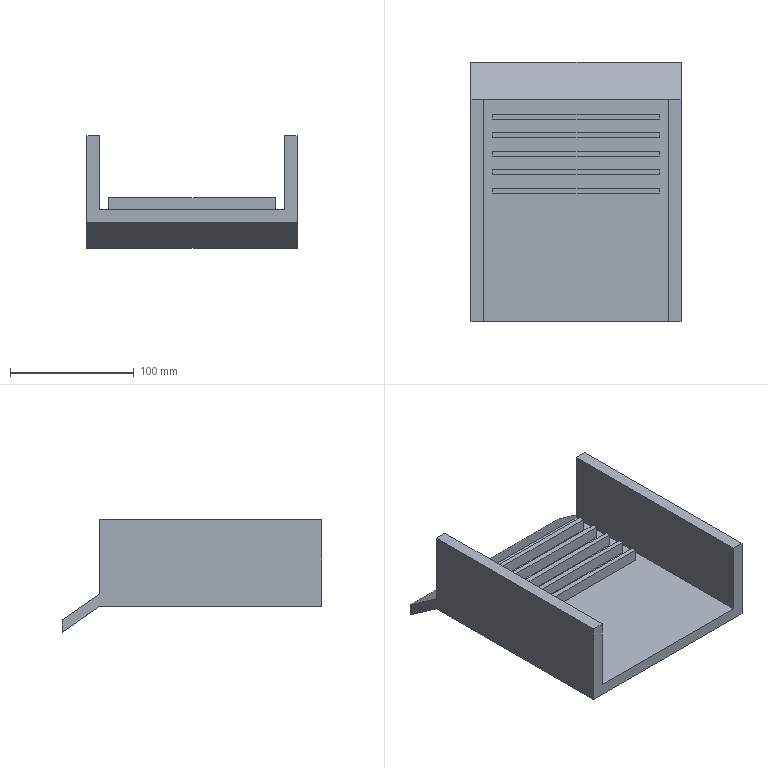Part | SolidWorks | features ICE 3, Extrusion 1, LPattern 1 | 1 solid | 39 faces | box 170 x 210 x 91.006 mm | volume 600000 mm3 | plane 39
STEP:
#1=CARTESIAN_POINT('',(67.5,14.,20.));
#2=VERTEX_POINT('',#1);
#3=CARTESIAN_POINT('',(67.5,18.,20.));
#4=VERTEX_POINT('',#3);
#5=CARTESIAN_POINT('',(67.5,14.,20.));
#6=DIRECTION('',(0.,1.,0.));
#7=VECTOR('',#6,1000.);
#8=LINE('',#5,#7);
#9=EDGE_CURVE('',#2,#4,#8,.T.);
#10=ORIENTED_EDGE('',*,*,#9,.T.);
#11=CARTESIAN_POINT('',(-67.5,18.,20.));
#12=VERTEX_POINT('',#11);
#13=CARTESIAN_POINT('',(-67.5,18.,20.));
#14=DIRECTION('',(-1.,0.,0.));
#15=VECTOR('',#14,1000.);
#16=LINE('',#13,#15);
#17=EDGE_CURVE('',#4,#12,#16,.T.);
#18=ORIENTED_EDGE('',*,*,#17,.T.);
#19=CARTESIAN_POINT('',(-67.5,14.,20.));
#20=VERTEX_POINT('',#19);
#21=CARTESIAN_POINT('',(-67.5,14.,20.));
#22=DIRECTION('',(0.,-1.,0.));
#23=VECTOR('',#22,1000.);
#24=LINE('',#21,#23);
#25=EDGE_CURVE('',#12,#20,#24,.T.);
#26=ORIENTED_EDGE('',*,*,#25,.T.);
#27=CARTESIAN_POINT('',(-67.5,14.,20.));
#28=DIRECTION('',(1.,0.,0.));
#29=VECTOR('',#28,1000.);
#30=LINE('',#27,#29);
#31=EDGE_CURVE('',#20,#2,#30,.T.);
#32=ORIENTED_EDGE('',*,*,#31,.T.);
#33=EDGE_LOOP('',(#10,#18,#26,#32));
#34=FACE_OUTER_BOUND('',#33,.T.);
#35=CARTESIAN_POINT('',(0.,-60.,20.));
#36=DIRECTION('',(0.,0.,-1.));
#37=DIRECTION('',(-1.,0.,0.));
#38=AXIS2_PLACEMENT_3D('',#35,#36,#37);
#39=PLANE('',#38);
#40=ADVANCED_FACE('',(#34),#39,.F.);
#41=CARTESIAN_POINT('',(-67.5,14.,10.));
#42=VERTEX_POINT('',#41);
#43=CARTESIAN_POINT('',(67.5,14.,10.));
#44=VERTEX_POINT('',#43);
#45=CARTESIAN_POINT('',(-67.5,14.,10.));
#46=DIRECTION('',(1.,0.,0.));
#47=VECTOR('',#46,1000.);
#48=LINE('',#45,#47);
#49=EDGE_CURVE('',#42,#44,#48,.T.);
#50=ORIENTED_EDGE('',*,*,#49,.T.);
#51=CARTESIAN_POINT('',(67.5,14.,20.));
#52=DIRECTION('',(0.,0.,-1.));
#53=VECTOR('',#52,1000.);
#54=LINE('',#51,#53);
#55=EDGE_CURVE('',#2,#44,#54,.T.);
#56=ORIENTED_EDGE('',*,*,#55,.F.);
#57=ORIENTED_EDGE('',*,*,#31,.F.);
#58=CARTESIAN_POINT('',(-67.5,14.,20.));
#59=DIRECTION('',(0.,0.,-1.));
#60=VECTOR('',#59,1000.);
#61=LINE('',#58,#60);
#62=EDGE_CURVE('',#20,#42,#61,.T.);
#63=ORIENTED_EDGE('',*,*,#62,.T.);
#64=EDGE_LOOP('',(#50,#56,#57,#63));
#65=FACE_OUTER_BOUND('',#64,.T.);
#66=CARTESIAN_POINT('',(-67.5,14.,20.));
#67=DIRECTION('',(0.,1.,0.));
#68=DIRECTION('',(0.,0.,1.));
#69=AXIS2_PLACEMENT_3D('',#66,#67,#68);
#70=PLANE('',#69);
#71=ADVANCED_FACE('',(#65),#70,.F.);
#72=CARTESIAN_POINT('',(-67.5,18.,10.));
#73=VERTEX_POINT('',#72);
#74=CARTESIAN_POINT('',(-67.5,14.,10.));
#75=DIRECTION('',(0.,-1.,0.));
#76=VECTOR('',#75,1000.);
#77=LINE('',#74,#76);
#78=EDGE_CURVE('',#73,#42,#77,.T.);
#79=ORIENTED_EDGE('',*,*,#78,.T.);
#80=ORIENTED_EDGE('',*,*,#62,.F.);
#81=ORIENTED_EDGE('',*,*,#25,.F.);
#82=CARTESIAN_POINT('',(-67.5,18.,20.));
#83=DIRECTION('',(0.,0.,-1.));
#84=VECTOR('',#83,1000.);
#85=LINE('',#82,#84);
#86=EDGE_CURVE('',#12,#73,#85,.T.);
#87=ORIENTED_EDGE('',*,*,#86,.T.);
#88=EDGE_LOOP('',(#79,#80,#81,#87));
#89=FACE_OUTER_BOUND('',#88,.T.);
#90=CARTESIAN_POINT('',(-67.5,14.,20.));
#91=DIRECTION('',(1.,0.,0.));
#92=DIRECTION('',(0.,0.,-1.));
#93=AXIS2_PLACEMENT_3D('',#90,#91,#92);
#94=PLANE('',#93);
#95=ADVANCED_FACE('',(#89),#94,.F.);
#96=CARTESIAN_POINT('',(67.5,18.,10.));
#97=VERTEX_POINT('',#96);
#98=CARTESIAN_POINT('',(-67.5,18.,10.));
#99=DIRECTION('',(-1.,0.,0.));
#100=VECTOR('',#99,1000.);
#101=LINE('',#98,#100);
#102=EDGE_CURVE('',#97,#73,#101,.T.);
#103=ORIENTED_EDGE('',*,*,#102,.T.);
#104=ORIENTED_EDGE('',*,*,#86,.F.);
#105=ORIENTED_EDGE('',*,*,#17,.F.);
#106=CARTESIAN_POINT('',(67.5,18.,20.));
#107=DIRECTION('',(0.,0.,-1.));
#108=VECTOR('',#107,1000.);
#109=LINE('',#106,#108);
#110=EDGE_CURVE('',#4,#97,#109,.T.);
#111=ORIENTED_EDGE('',*,*,#110,.T.);
#112=EDGE_LOOP('',(#103,#104,#105,#111));
#113=FACE_OUTER_BOUND('',#112,.T.);
#114=CARTESIAN_POINT('',(-67.5,18.,20.));
#115=DIRECTION('',(0.,-1.,0.));
#116=DIRECTION('',(0.,0.,-1.));
#117=AXIS2_PLACEMENT_3D('',#114,#115,#116);
#118=PLANE('',#117);
#119=ADVANCED_FACE('',(#113),#118,.F.);
#120=CARTESIAN_POINT('',(67.5,14.,10.));
#121=DIRECTION('',(0.,1.,0.));
#122=VECTOR('',#121,1000.);
#123=LINE('',#120,#122);
#124=EDGE_CURVE('',#44,#97,#123,.T.);
#125=ORIENTED_EDGE('',*,*,#124,.T.);
#126=ORIENTED_EDGE('',*,*,#110,.F.);
#127=ORIENTED_EDGE('',*,*,#9,.F.);
#128=ORIENTED_EDGE('',*,*,#55,.T.);
#129=EDGE_LOOP('',(#125,#126,#127,#128));
#130=FACE_OUTER_BOUND('',#129,.T.);
#131=CARTESIAN_POINT('',(67.5,14.,20.));
#132=DIRECTION('',(-1.,0.,0.));
#133=DIRECTION('',(0.,0.,1.));
#134=AXIS2_PLACEMENT_3D('',#131,#132,#133);
#135=PLANE('',#134);
#136=ADVANCED_FACE('',(#130),#135,.F.);
#137=CARTESIAN_POINT('',(67.5,29.,20.));
#138=VERTEX_POINT('',#137);
#139=CARTESIAN_POINT('',(67.5,33.,20.));
#140=VERTEX_POINT('',#139);
#141=CARTESIAN_POINT('',(67.5,29.,20.));
#142=DIRECTION('',(0.,1.,0.));
#143=VECTOR('',#142,1000.);
#144=LINE('',#141,#143);
#145=EDGE_CURVE('',#138,#140,#144,.T.);
#146=ORIENTED_EDGE('',*,*,#145,.T.);
#147=CARTESIAN_POINT('',(-67.5,33.,20.));
#148=VERTEX_POINT('',#147);
#149=CARTESIAN_POINT('',(-67.5,33.,20.));
#150=DIRECTION('',(-1.,0.,0.));
#151=VECTOR('',#150,1000.);
#152=LINE('',#149,#151);
#153=EDGE_CURVE('',#140,#148,#152,.T.);
#154=ORIENTED_EDGE('',*,*,#153,.T.);
#155=CARTESIAN_POINT('',(-67.5,29.,20.));
#156=VERTEX_POINT('',#155);
#157=CARTESIAN_POINT('',(-67.5,29.,20.));
#158=DIRECTION('',(0.,-1.,0.));
#159=VECTOR('',#158,1000.);
#160=LINE('',#157,#159);
#161=EDGE_CURVE('',#148,#156,#160,.T.);
#162=ORIENTED_EDGE('',*,*,#161,.T.);
#163=CARTESIAN_POINT('',(-67.5,29.,20.));
#164=DIRECTION('',(1.,0.,0.));
#165=VECTOR('',#164,1000.);
#166=LINE('',#163,#165);
#167=EDGE_CURVE('',#156,#138,#166,.T.);
#168=ORIENTED_EDGE('',*,*,#167,.T.);
#169=EDGE_LOOP('',(#146,#154,#162,#168));
#170=FACE_OUTER_BOUND('',#169,.T.);
#171=CARTESIAN_POINT('',(0.,-45.,20.));
#172=DIRECTION('',(0.,0.,-1.));
#173=DIRECTION('',(-1.,0.,0.));
#174=AXIS2_PLACEMENT_3D('',#171,#172,#173);
#175=PLANE('',#174);
#176=ADVANCED_FACE('',(#170),#175,.F.);
#177=CARTESIAN_POINT('',(-67.5,29.,10.));
#178=VERTEX_POINT('',#177);
#179=CARTESIAN_POINT('',(67.5,29.,10.));
#180=VERTEX_POINT('',#179);
#181=CARTESIAN_POINT('',(-67.5,29.,10.));
#182=DIRECTION('',(1.,0.,0.));
#183=VECTOR('',#182,1000.);
#184=LINE('',#181,#183);
#185=EDGE_CURVE('',#178,#180,#184,.T.);
#186=ORIENTED_EDGE('',*,*,#185,.T.);
#187=CARTESIAN_POINT('',(67.5,29.,20.));
#188=DIRECTION('',(0.,0.,-1.));
#189=VECTOR('',#188,1000.);
#190=LINE('',#187,#189);
#191=EDGE_CURVE('',#138,#180,#190,.T.);
#192=ORIENTED_EDGE('',*,*,#191,.F.);
#193=ORIENTED_EDGE('',*,*,#167,.F.);
#194=CARTESIAN_POINT('',(-67.5,29.,20.));
#195=DIRECTION('',(0.,0.,-1.));
#196=VECTOR('',#195,1000.);
#197=LINE('',#194,#196);
#198=EDGE_CURVE('',#156,#178,#197,.T.);
#199=ORIENTED_EDGE('',*,*,#198,.T.);
#200=EDGE_LOOP('',(#186,#192,#193,#199));
#201=FACE_OUTER_BOUND('',#200,.T.);
#202=CARTESIAN_POINT('',(-67.5,29.,20.));
#203=DIRECTION('',(0.,1.,0.));
#204=DIRECTION('',(0.,0.,1.));
#205=AXIS2_PLACEMENT_3D('',#202,#203,#204);
#206=PLANE('',#205);
#207=ADVANCED_FACE('',(#201),#206,.F.);
#208=CARTESIAN_POINT('',(-67.5,33.,10.));
#209=VERTEX_POINT('',#208);
#210=CARTESIAN_POINT('',(-67.5,29.,10.));
#211=DIRECTION('',(0.,-1.,0.));
#212=VECTOR('',#211,1000.);
#213=LINE('',#210,#212);
#214=EDGE_CURVE('',#209,#178,#213,.T.);
#215=ORIENTED_EDGE('',*,*,#214,.T.);
#216=ORIENTED_EDGE('',*,*,#198,.F.);
#217=ORIENTED_EDGE('',*,*,#161,.F.);
#218=CARTESIAN_POINT('',(-67.5,33.,20.));
#219=DIRECTION('',(0.,0.,-1.));
#220=VECTOR('',#219,1000.);
#221=LINE('',#218,#220);
#222=EDGE_CURVE('',#148,#209,#221,.T.);
#223=ORIENTED_EDGE('',*,*,#222,.T.);
#224=EDGE_LOOP('',(#215,#216,#217,#223));
#225=FACE_OUTER_BOUND('',#224,.T.);
#226=CARTESIAN_POINT('',(-67.5,29.,20.));
#227=DIRECTION('',(1.,0.,0.));
#228=DIRECTION('',(0.,0.,-1.));
#229=AXIS2_PLACEMENT_3D('',#226,#227,#228);
#230=PLANE('',#229);
#231=ADVANCED_FACE('',(#225),#230,.F.);
#232=CARTESIAN_POINT('',(67.5,33.,10.));
#233=VERTEX_POINT('',#232);
#234=CARTESIAN_POINT('',(-67.5,33.,10.));
#235=DIRECTION('',(-1.,0.,0.));
#236=VECTOR('',#235,1000.);
#237=LINE('',#234,#236);
#238=EDGE_CURVE('',#233,#209,#237,.T.);
#239=ORIENTED_EDGE('',*,*,#238,.T.);
#240=ORIENTED_EDGE('',*,*,#222,.F.);
#241=ORIENTED_EDGE('',*,*,#153,.F.);
#242=CARTESIAN_POINT('',(67.5,33.,20.));
#243=DIRECTION('',(0.,0.,-1.));
#244=VECTOR('',#243,1000.);
#245=LINE('',#242,#244);
#246=EDGE_CURVE('',#140,#233,#245,.T.);
#247=ORIENTED_EDGE('',*,*,#246,.T.);
#248=EDGE_LOOP('',(#239,#240,#241,#247));
#249=FACE_OUTER_BOUND('',#248,.T.);
#250=CARTESIAN_POINT('',(-67.5,33.,20.));
#251=DIRECTION('',(0.,-1.,0.));
#252=DIRECTION('',(0.,0.,-1.));
#253=AXIS2_PLACEMENT_3D('',#250,#251,#252);
#254=PLANE('',#253);
#255=ADVANCED_FACE('',(#249),#254,.F.);
#256=CARTESIAN_POINT('',(67.5,29.,10.));
#257=DIRECTION('',(0.,1.,0.));
#258=VECTOR('',#257,1000.);
#259=LINE('',#256,#258);
#260=EDGE_CURVE('',#180,#233,#259,.T.);
#261=ORIENTED_EDGE('',*,*,#260,.T.);
#262=ORIENTED_EDGE('',*,*,#246,.F.);
#263=ORIENTED_EDGE('',*,*,#145,.F.);
#264=ORIENTED_EDGE('',*,*,#191,.T.);
#265=EDGE_LOOP('',(#261,#262,#263,#264));
#266=FACE_OUTER_BOUND('',#265,.T.);
#267=CARTESIAN_POINT('',(67.5,29.,20.));
#268=DIRECTION('',(-1.,0.,0.));
#269=DIRECTION('',(0.,0.,1.));
#270=AXIS2_PLACEMENT_3D('',#267,#268,#269);
#271=PLANE('',#270);
#272=ADVANCED_FACE('',(#266),#271,.F.);
#273=CARTESIAN_POINT('',(67.5,44.,20.));
#274=VERTEX_POINT('',#273);
#275=CARTESIAN_POINT('',(67.5,48.,20.));
#276=VERTEX_POINT('',#275);
#277=CARTESIAN_POINT('',(67.5,44.,20.));
#278=DIRECTION('',(0.,1.,0.));
#279=VECTOR('',#278,1000.);
#280=LINE('',#277,#279);
#281=EDGE_CURVE('',#274,#276,#280,.T.);
#282=ORIENTED_EDGE('',*,*,#281,.T.);
#283=CARTESIAN_POINT('',(-67.5,48.,20.));
#284=VERTEX_POINT('',#283);
#285=CARTESIAN_POINT('',(-67.5,48.,20.));
#286=DIRECTION('',(-1.,0.,0.));
#287=VECTOR('',#286,1000.);
#288=LINE('',#285,#287);
#289=EDGE_CURVE('',#276,#284,#288,.T.);
#290=ORIENTED_EDGE('',*,*,#289,.T.);
#291=CARTESIAN_POINT('',(-67.5,44.,20.));
#292=VERTEX_POINT('',#291);
#293=CARTESIAN_POINT('',(-67.5,44.,20.));
#294=DIRECTION('',(0.,-1.,0.));
#295=VECTOR('',#294,1000.);
#296=LINE('',#293,#295);
#297=EDGE_CURVE('',#284,#292,#296,.T.);
#298=ORIENTED_EDGE('',*,*,#297,.T.);
#299=CARTESIAN_POINT('',(-67.5,44.,20.));
#300=DIRECTION('',(1.,0.,0.));
#301=VECTOR('',#300,1000.);
#302=LINE('',#299,#301);
#303=EDGE_CURVE('',#292,#274,#302,.T.);
#304=ORIENTED_EDGE('',*,*,#303,.T.);
#305=EDGE_LOOP('',(#282,#290,#298,#304));
#306=FACE_OUTER_BOUND('',#305,.T.);
#307=CARTESIAN_POINT('',(0.,-30.,20.));
#308=DIRECTION('',(0.,0.,-1.));
#309=DIRECTION('',(-1.,0.,0.));
#310=AXIS2_PLACEMENT_3D('',#307,#308,#309);
#311=PLANE('',#310);
#312=ADVANCED_FACE('',(#306),#311,.F.);
#313=CARTESIAN_POINT('',(-67.5,44.,10.));
#314=VERTEX_POINT('',#313);
#315=CARTESIAN_POINT('',(67.5,44.,10.));
#316=VERTEX_POINT('',#315);
#317=CARTESIAN_POINT('',(-67.5,44.,10.));
#318=DIRECTION('',(1.,0.,0.));
#319=VECTOR('',#318,1000.);
#320=LINE('',#317,#319);
#321=EDGE_CURVE('',#314,#316,#320,.T.);
#322=ORIENTED_EDGE('',*,*,#321,.T.);
#323=CARTESIAN_POINT('',(67.5,44.,20.));
#324=DIRECTION('',(0.,0.,-1.));
#325=VECTOR('',#324,1000.);
#326=LINE('',#323,#325);
#327=EDGE_CURVE('',#274,#316,#326,.T.);
#328=ORIENTED_EDGE('',*,*,#327,.F.);
#329=ORIENTED_EDGE('',*,*,#303,.F.);
#330=CARTESIAN_POINT('',(-67.5,44.,20.));
#331=DIRECTION('',(0.,0.,-1.));
#332=VECTOR('',#331,1000.);
#333=LINE('',#330,#332);
#334=EDGE_CURVE('',#292,#314,#333,.T.);
#335=ORIENTED_EDGE('',*,*,#334,.T.);
#336=EDGE_LOOP('',(#322,#328,#329,#335));
#337=FACE_OUTER_BOUND('',#336,.T.);
#338=CARTESIAN_POINT('',(-67.5,44.,20.));
#339=DIRECTION('',(0.,1.,0.));
#340=DIRECTION('',(0.,0.,1.));
#341=AXIS2_PLACEMENT_3D('',#338,#339,#340);
#342=PLANE('',#341);
#343=ADVANCED_FACE('',(#337),#342,.F.);
#344=CARTESIAN_POINT('',(-67.5,48.,10.));
#345=VERTEX_POINT('',#344);
#346=CARTESIAN_POINT('',(-67.5,44.,10.));
#347=DIRECTION('',(0.,-1.,0.));
#348=VECTOR('',#347,1000.);
#349=LINE('',#346,#348);
#350=EDGE_CURVE('',#345,#314,#349,.T.);
#351=ORIENTED_EDGE('',*,*,#350,.T.);
#352=ORIENTED_EDGE('',*,*,#334,.F.);
#353=ORIENTED_EDGE('',*,*,#297,.F.);
#354=CARTESIAN_POINT('',(-67.5,48.,20.));
#355=DIRECTION('',(0.,0.,-1.));
#356=VECTOR('',#355,1000.);
#357=LINE('',#354,#356);
#358=EDGE_CURVE('',#284,#345,#357,.T.);
#359=ORIENTED_EDGE('',*,*,#358,.T.);
#360=EDGE_LOOP('',(#351,#352,#353,#359));
#361=FACE_OUTER_BOUND('',#360,.T.);
#362=CARTESIAN_POINT('',(-67.5,44.,20.));
#363=DIRECTION('',(1.,0.,0.));
#364=DIRECTION('',(0.,0.,-1.));
#365=AXIS2_PLACEMENT_3D('',#362,#363,#364);
#366=PLANE('',#365);
#367=ADVANCED_FACE('',(#361),#366,.F.);
#368=CARTESIAN_POINT('',(67.5,48.,10.));
#369=VERTEX_POINT('',#368);
#370=CARTESIAN_POINT('',(-67.5,48.,10.));
#371=DIRECTION('',(-1.,0.,0.));
#372=VECTOR('',#371,1000.);
#373=LINE('',#370,#372);
#374=EDGE_CURVE('',#369,#345,#373,.T.);
#375=ORIENTED_EDGE('',*,*,#374,.T.);
#376=ORIENTED_EDGE('',*,*,#358,.F.);
#377=ORIENTED_EDGE('',*,*,#289,.F.);
#378=CARTESIAN_POINT('',(67.5,48.,20.));
#379=DIRECTION('',(0.,0.,-1.));
#380=VECTOR('',#379,1000.);
#381=LINE('',#378,#380);
#382=EDGE_CURVE('',#276,#369,#381,.T.);
#383=ORIENTED_EDGE('',*,*,#382,.T.);
#384=EDGE_LOOP('',(#375,#376,#377,#383));
#385=FACE_OUTER_BOUND('',#384,.T.);
#386=CARTESIAN_POINT('',(-67.5,48.,20.));
#387=DIRECTION('',(0.,-1.,0.));
#388=DIRECTION('',(0.,0.,-1.));
#389=AXIS2_PLACEMENT_3D('',#386,#387,#388);
#390=PLANE('',#389);
#391=ADVANCED_FACE('',(#385),#390,.F.);
#392=CARTESIAN_POINT('',(67.5,44.,10.));
#393=DIRECTION('',(0.,1.,0.));
#394=VECTOR('',#393,1000.);
#395=LINE('',#392,#394);
#396=EDGE_CURVE('',#316,#369,#395,.T.);
#397=ORIENTED_EDGE('',*,*,#396,.T.);
#398=ORIENTED_EDGE('',*,*,#382,.F.);
#399=ORIENTED_EDGE('',*,*,#281,.F.);
#400=ORIENTED_EDGE('',*,*,#327,.T.);
#401=EDGE_LOOP('',(#397,#398,#399,#400));
#402=FACE_OUTER_BOUND('',#401,.T.);
#403=CARTESIAN_POINT('',(67.5,44.,20.));
#404=DIRECTION('',(-1.,0.,0.));
#405=DIRECTION('',(0.,0.,1.));
#406=AXIS2_PLACEMENT_3D('',#403,#404,#405);
#407=PLANE('',#406);
#408=ADVANCED_FACE('',(#402),#407,.F.);
#409=CARTESIAN_POINT('',(67.5,74.,10.));
#410=VERTEX_POINT('',#409);
#411=CARTESIAN_POINT('',(67.5,78.,10.));
#412=VERTEX_POINT('',#411);
#413=CARTESIAN_POINT('',(67.5,74.,10.));
#414=DIRECTION('',(0.,1.,0.));
#415=VECTOR('',#414,1000.);
#416=LINE('',#413,#415);
#417=EDGE_CURVE('',#410,#412,#416,.T.);
#418=ORIENTED_EDGE('',*,*,#417,.F.);
#419=CARTESIAN_POINT('',(-67.5,74.,10.));
#420=VERTEX_POINT('',#419);
#421=CARTESIAN_POINT('',(-67.5,74.,10.));
#422=DIRECTION('',(1.,0.,0.));
#423=VECTOR('',#422,1000.);
#424=LINE('',#421,#423);
#425=EDGE_CURVE('',#420,#410,#424,.T.);
#426=ORIENTED_EDGE('',*,*,#425,.F.);
#427=CARTESIAN_POINT('',(-67.5,78.,10.));
#428=VERTEX_POINT('',#427);
#429=CARTESIAN_POINT('',(-67.5,74.,10.));
#430=DIRECTION('',(0.,-1.,0.));
#431=VECTOR('',#430,1000.);
#432=LINE('',#429,#431);
#433=EDGE_CURVE('',#428,#420,#432,.T.);
#434=ORIENTED_EDGE('',*,*,#433,.F.);
#435=CARTESIAN_POINT('',(-67.5,78.,10.));
#436=DIRECTION('',(-1.,0.,0.));
#437=VECTOR('',#436,1000.);
#438=LINE('',#435,#437);
#439=EDGE_CURVE('',#412,#428,#438,.T.);
#440=ORIENTED_EDGE('',*,*,#439,.F.);
#441=EDGE_LOOP('',(#418,#426,#434,#440));
#442=FACE_BOUND('',#441,.T.);
#443=CARTESIAN_POINT('',(75.,90.,10.));
#444=VERTEX_POINT('',#443);
#445=CARTESIAN_POINT('',(75.,-90.,10.));
#446=VERTEX_POINT('',#445);
#447=CARTESIAN_POINT('',(75.,90.,10.));
#448=DIRECTION('',(0.,-1.,0.));
#449=VECTOR('',#448,1000.);
#450=LINE('',#447,#449);
#451=EDGE_CURVE('',#444,#446,#450,.T.);
#452=ORIENTED_EDGE('',*,*,#451,.F.);
#453=CARTESIAN_POINT('',(-75.,90.,10.));
#454=VERTEX_POINT('',#453);
#455=CARTESIAN_POINT('',(-85.,90.,10.));
#456=DIRECTION('',(-1.,0.,0.));
#457=VECTOR('',#456,1000.);
#458=LINE('',#455,#457);
#459=EDGE_CURVE('',#444,#454,#458,.T.);
#460=ORIENTED_EDGE('',*,*,#459,.T.);
#461=CARTESIAN_POINT('',(-75.,-90.,10.));
#462=VERTEX_POINT('',#461);
#463=CARTESIAN_POINT('',(-75.,90.,10.));
#464=DIRECTION('',(0.,1.,0.));
#465=VECTOR('',#464,1000.);
#466=LINE('',#463,#465);
#467=EDGE_CURVE('',#462,#454,#466,.T.);
#468=ORIENTED_EDGE('',*,*,#467,.F.);
#469=CARTESIAN_POINT('',(-85.,-90.,10.));
#470=DIRECTION('',(1.,0.,0.));
#471=VECTOR('',#470,1000.);
#472=LINE('',#469,#471);
#473=EDGE_CURVE('',#462,#446,#472,.T.);
#474=ORIENTED_EDGE('',*,*,#473,.T.);
#475=EDGE_LOOP('',(#452,#460,#468,#474));
#476=FACE_OUTER_BOUND('',#475,.T.);
#477=CARTESIAN_POINT('',(67.5,59.,10.));
#478=VERTEX_POINT('',#477);
#479=CARTESIAN_POINT('',(67.5,63.,10.));
#480=VERTEX_POINT('',#479);
#481=CARTESIAN_POINT('',(67.5,59.,10.));
#482=DIRECTION('',(0.,1.,0.));
#483=VECTOR('',#482,1000.);
#484=LINE('',#481,#483);
#485=EDGE_CURVE('',#478,#480,#484,.T.);
#486=ORIENTED_EDGE('',*,*,#485,.F.);
#487=CARTESIAN_POINT('',(-67.5,59.,10.));
#488=VERTEX_POINT('',#487);
#489=CARTESIAN_POINT('',(-67.5,59.,10.));
#490=DIRECTION('',(1.,0.,0.));
#491=VECTOR('',#490,1000.);
#492=LINE('',#489,#491);
#493=EDGE_CURVE('',#488,#478,#492,.T.);
#494=ORIENTED_EDGE('',*,*,#493,.F.);
#495=CARTESIAN_POINT('',(-67.5,63.,10.));
#496=VERTEX_POINT('',#495);
#497=CARTESIAN_POINT('',(-67.5,59.,10.));
#498=DIRECTION('',(0.,-1.,0.));
#499=VECTOR('',#498,1000.);
#500=LINE('',#497,#499);
#501=EDGE_CURVE('',#496,#488,#500,.T.);
#502=ORIENTED_EDGE('',*,*,#501,.F.);
#503=CARTESIAN_POINT('',(-67.5,63.,10.));
#504=DIRECTION('',(-1.,0.,0.));
#505=VECTOR('',#504,1000.);
#506=LINE('',#503,#505);
#507=EDGE_CURVE('',#480,#496,#506,.T.);
#508=ORIENTED_EDGE('',*,*,#507,.F.);
#509=EDGE_LOOP('',(#486,#494,#502,#508));
#510=FACE_BOUND('',#509,.T.);
#511=ORIENTED_EDGE('',*,*,#396,.F.);
#512=ORIENTED_EDGE('',*,*,#321,.F.);
#513=ORIENTED_EDGE('',*,*,#350,.F.);
#514=ORIENTED_EDGE('',*,*,#374,.F.);
#515=EDGE_LOOP('',(#511,#512,#513,#514));
#516=FACE_BOUND('',#515,.T.);
#517=ORIENTED_EDGE('',*,*,#260,.F.);
#518=ORIENTED_EDGE('',*,*,#185,.F.);
#519=ORIENTED_EDGE('',*,*,#214,.F.);
#520=ORIENTED_EDGE('',*,*,#238,.F.);
#521=EDGE_LOOP('',(#517,#518,#519,#520));
#522=FACE_BOUND('',#521,.T.);
#523=ORIENTED_EDGE('',*,*,#124,.F.);
#524=ORIENTED_EDGE('',*,*,#49,.F.);
#525=ORIENTED_EDGE('',*,*,#78,.F.);
#526=ORIENTED_EDGE('',*,*,#102,.F.);
#527=EDGE_LOOP('',(#523,#524,#525,#526));
#528=FACE_BOUND('',#527,.T.);
#529=CARTESIAN_POINT('',(0.,0.,10.));
#530=DIRECTION('',(0.,0.,-1.));
#531=DIRECTION('',(-1.,0.,0.));
#532=AXIS2_PLACEMENT_3D('',#529,#530,#531);
#533=PLANE('',#532);
#534=ADVANCED_FACE('',(#442,#476,#510,#516,#522,#528),#533,.F.);
#535=CARTESIAN_POINT('',(-85.,90.,10.));
#536=VERTEX_POINT('',#535);
#537=CARTESIAN_POINT('',(-128.144,90.,10.));
#538=DIRECTION('',(1.,0.,0.));
#539=VECTOR('',#538,1000.);
#540=LINE('',#537,#539);
#541=EDGE_CURVE('',#536,#454,#540,.T.);
#542=ORIENTED_EDGE('',*,*,#541,.F.);
#543=CARTESIAN_POINT('',(-85.,90.,70.));
#544=VERTEX_POINT('',#543);
#545=CARTESIAN_POINT('',(-85.,90.,10.));
#546=DIRECTION('',(0.,0.,-1.));
#547=VECTOR('',#546,1000.);
#548=LINE('',#545,#547);
#549=EDGE_CURVE('',#544,#536,#548,.T.);
#550=ORIENTED_EDGE('',*,*,#549,.F.);
#551=CARTESIAN_POINT('',(-75.,90.,70.));
#552=VERTEX_POINT('',#551);
#553=CARTESIAN_POINT('',(-85.,90.,70.));
#554=DIRECTION('',(-1.,0.,0.));
#555=VECTOR('',#554,1000.);
#556=LINE('',#553,#555);
#557=EDGE_CURVE('',#552,#544,#556,.T.);
#558=ORIENTED_EDGE('',*,*,#557,.F.);
#559=CARTESIAN_POINT('',(-75.,90.,70.));
#560=DIRECTION('',(0.,0.,-1.));
#561=VECTOR('',#560,1000.);
#562=LINE('',#559,#561);
#563=EDGE_CURVE('',#552,#454,#562,.T.);
#564=ORIENTED_EDGE('',*,*,#563,.T.);
#565=EDGE_LOOP('',(#542,#550,#558,#564));
#566=FACE_OUTER_BOUND('',#565,.T.);
#567=CARTESIAN_POINT('',(-85.,90.,10.));
#568=DIRECTION('',(0.,-1.,0.));
#569=DIRECTION('',(0.,0.,-1.));
#570=AXIS2_PLACEMENT_3D('',#567,#568,#569);
#571=PLANE('',#570);
#572=ADVANCED_FACE('',(#566),#571,.F.);
#573=CARTESIAN_POINT('',(85.,90.,10.));
#574=VERTEX_POINT('',#573);
#575=CARTESIAN_POINT('',(-128.144,90.,10.));
#576=DIRECTION('',(1.,0.,0.));
#577=VECTOR('',#576,1000.);
#578=LINE('',#575,#577);
#579=EDGE_CURVE('',#444,#574,#578,.T.);
#580=ORIENTED_EDGE('',*,*,#579,.F.);
#581=CARTESIAN_POINT('',(75.,90.,70.));
#582=VERTEX_POINT('',#581);
#583=CARTESIAN_POINT('',(75.,90.,70.));
#584=DIRECTION('',(0.,0.,-1.));
#585=VECTOR('',#584,1000.);
#586=LINE('',#583,#585);
#587=EDGE_CURVE('',#582,#444,#586,.T.);
#588=ORIENTED_EDGE('',*,*,#587,.F.);
#589=CARTESIAN_POINT('',(85.,90.,70.));
#590=VERTEX_POINT('',#589);
#591=CARTESIAN_POINT('',(85.,90.,70.));
#592=DIRECTION('',(-1.,0.,0.));
#593=VECTOR('',#592,1000.);
#594=LINE('',#591,#593);
#595=EDGE_CURVE('',#590,#582,#594,.T.);
#596=ORIENTED_EDGE('',*,*,#595,.F.);
#597=CARTESIAN_POINT('',(85.,90.,10.));
#598=DIRECTION('',(0.,0.,-1.));
#599=VECTOR('',#598,1000.);
#600=LINE('',#597,#599);
#601=EDGE_CURVE('',#590,#574,#600,.T.);
#602=ORIENTED_EDGE('',*,*,#601,.T.);
#603=EDGE_LOOP('',(#580,#588,#596,#602));
#604=FACE_OUTER_BOUND('',#603,.T.);
#605=CARTESIAN_POINT('',(-85.,90.,10.));
#606=DIRECTION('',(0.,-1.,0.));
#607=DIRECTION('',(0.,0.,-1.));
#608=AXIS2_PLACEMENT_3D('',#605,#606,#607);
#609=PLANE('',#608);
#610=ADVANCED_FACE('',(#604),#609,.F.);
#611=CARTESIAN_POINT('',(85.,-90.,0.));
#612=VERTEX_POINT('',#611);
#613=CARTESIAN_POINT('',(85.,90.,0.));
#614=VERTEX_POINT('',#613);
#615=CARTESIAN_POINT('',(85.,-90.,0.));
#616=DIRECTION('',(0.,1.,0.));
#617=VECTOR('',#616,1000.);
#618=LINE('',#615,#617);
#619=EDGE_CURVE('',#612,#614,#618,.T.);
#620=ORIENTED_EDGE('',*,*,#619,.T.);
#621=CARTESIAN_POINT('',(85.,120.,-21.006));
#622=VERTEX_POINT('',#621);
#623=CARTESIAN_POINT('',(85.,90.,0.));
#624=DIRECTION('',(0.,0.8192,-0.5736));
#625=VECTOR('',#624,1000.);
#626=LINE('',#623,#625);
#627=EDGE_CURVE('',#614,#622,#626,.T.);
#628=ORIENTED_EDGE('',*,*,#627,.T.);
#629=CARTESIAN_POINT('',(85.,120.,-11.006));
#630=VERTEX_POINT('',#629);
#631=CARTESIAN_POINT('',(85.,120.,-21.006));
#632=DIRECTION('',(0.,0.,1.));
#633=VECTOR('',#632,1000.);
#634=LINE('',#631,#633);
#635=EDGE_CURVE('',#622,#630,#634,.T.);
#636=ORIENTED_EDGE('',*,*,#635,.T.);
#637=CARTESIAN_POINT('',(85.,120.,-11.006));
#638=DIRECTION('',(0.,-0.8192,0.5736));
#639=VECTOR('',#638,1000.);
#640=LINE('',#637,#639);
#641=EDGE_CURVE('',#630,#574,#640,.T.);
#642=ORIENTED_EDGE('',*,*,#641,.T.);
#643=ORIENTED_EDGE('',*,*,#601,.F.);
#644=CARTESIAN_POINT('',(85.,-90.,70.));
#645=VERTEX_POINT('',#644);
#646=CARTESIAN_POINT('',(85.,90.,70.));
#647=DIRECTION('',(0.,1.,0.));
#648=VECTOR('',#647,1000.);
#649=LINE('',#646,#648);
#650=EDGE_CURVE('',#645,#590,#649,.T.);
#651=ORIENTED_EDGE('',*,*,#650,.F.);
#652=CARTESIAN_POINT('',(85.,-90.,10.));
#653=DIRECTION('',(0.,0.,-1.));
#654=VECTOR('',#653,1000.);
#655=LINE('',#652,#654);
#656=EDGE_CURVE('',#645,#612,#655,.T.);
#657=ORIENTED_EDGE('',*,*,#656,.T.);
#658=EDGE_LOOP('',(#620,#628,#636,#642,#643,#651,#657));
#659=FACE_OUTER_BOUND('',#658,.T.);
#660=CARTESIAN_POINT('',(85.,-90.,10.));
#661=DIRECTION('',(-1.,0.,0.));
#662=DIRECTION('',(0.,0.,1.));
#663=AXIS2_PLACEMENT_3D('',#660,#661,#662);
#664=PLANE('',#663);
#665=ADVANCED_FACE('',(#659),#664,.F.);
#666=CARTESIAN_POINT('',(-85.,90.,0.));
#667=VERTEX_POINT('',#666);
#668=CARTESIAN_POINT('',(-85.,-90.,0.));
#669=VERTEX_POINT('',#668);
#670=CARTESIAN_POINT('',(-85.,-90.,0.));
#671=DIRECTION('',(0.,-1.,0.));
#672=VECTOR('',#671,1000.);
#673=LINE('',#670,#672);
#674=EDGE_CURVE('',#667,#669,#673,.T.);
#675=ORIENTED_EDGE('',*,*,#674,.T.);
#676=CARTESIAN_POINT('',(-85.,-90.,70.));
#677=VERTEX_POINT('',#676);
#678=CARTESIAN_POINT('',(-85.,-90.,10.));
#679=DIRECTION('',(0.,0.,-1.));
#680=VECTOR('',#679,1000.);
#681=LINE('',#678,#680);
#682=EDGE_CURVE('',#677,#669,#681,.T.);
#683=ORIENTED_EDGE('',*,*,#682,.F.);
#684=CARTESIAN_POINT('',(-85.,90.,70.));
#685=DIRECTION('',(0.,-1.,0.));
#686=VECTOR('',#685,1000.);
#687=LINE('',#684,#686);
#688=EDGE_CURVE('',#544,#677,#687,.T.);
#689=ORIENTED_EDGE('',*,*,#688,.F.);
#690=ORIENTED_EDGE('',*,*,#549,.T.);
#691=CARTESIAN_POINT('',(-85.,120.,-11.006));
#692=VERTEX_POINT('',#691);
#693=CARTESIAN_POINT('',(-85.,120.,-11.006));
#694=DIRECTION('',(0.,0.8192,-0.5736));
#695=VECTOR('',#694,1000.);
#696=LINE('',#693,#695);
#697=EDGE_CURVE('',#536,#692,#696,.T.);
#698=ORIENTED_EDGE('',*,*,#697,.T.);
#699=CARTESIAN_POINT('',(-85.,120.,-21.006));
#700=VERTEX_POINT('',#699);
#701=CARTESIAN_POINT('',(-85.,120.,-21.006));
#702=DIRECTION('',(0.,0.,-1.));
#703=VECTOR('',#702,1000.);
#704=LINE('',#701,#703);
#705=EDGE_CURVE('',#692,#700,#704,.T.);
#706=ORIENTED_EDGE('',*,*,#705,.T.);
#707=CARTESIAN_POINT('',(-85.,90.,0.));
#708=DIRECTION('',(0.,-0.8192,0.5736));
#709=VECTOR('',#708,1000.);
#710=LINE('',#707,#709);
#711=EDGE_CURVE('',#700,#667,#710,.T.);
#712=ORIENTED_EDGE('',*,*,#711,.T.);
#713=EDGE_LOOP('',(#675,#683,#689,#690,#698,#706,#712));
#714=FACE_OUTER_BOUND('',#713,.T.);
#715=CARTESIAN_POINT('',(-85.,-90.,10.));
#716=DIRECTION('',(1.,0.,0.));
#717=DIRECTION('',(0.,0.,-1.));
#718=AXIS2_PLACEMENT_3D('',#715,#716,#717);
#719=PLANE('',#718);
#720=ADVANCED_FACE('',(#714),#719,.F.);
#721=CARTESIAN_POINT('',(-85.,-90.,0.));
#722=DIRECTION('',(1.,0.,0.));
#723=VECTOR('',#722,1000.);
#724=LINE('',#721,#723);
#725=EDGE_CURVE('',#669,#612,#724,.T.);
#726=ORIENTED_EDGE('',*,*,#725,.T.);
#727=ORIENTED_EDGE('',*,*,#656,.F.);
#728=CARTESIAN_POINT('',(75.,-90.,70.));
#729=VERTEX_POINT('',#728);
#730=CARTESIAN_POINT('',(85.,-90.,70.));
#731=DIRECTION('',(1.,0.,0.));
#732=VECTOR('',#731,1000.);
#733=LINE('',#730,#732);
#734=EDGE_CURVE('',#729,#645,#733,.T.);
#735=ORIENTED_EDGE('',*,*,#734,.F.);
#736=CARTESIAN_POINT('',(75.,-90.,70.));
#737=DIRECTION('',(0.,0.,-1.));
#738=VECTOR('',#737,1000.);
#739=LINE('',#736,#738);
#740=EDGE_CURVE('',#729,#446,#739,.T.);
#741=ORIENTED_EDGE('',*,*,#740,.T.);
#742=ORIENTED_EDGE('',*,*,#473,.F.);
#743=CARTESIAN_POINT('',(-75.,-90.,70.));
#744=VERTEX_POINT('',#743);
#745=CARTESIAN_POINT('',(-75.,-90.,70.));
#746=DIRECTION('',(0.,0.,-1.));
#747=VECTOR('',#746,1000.);
#748=LINE('',#745,#747);
#749=EDGE_CURVE('',#744,#462,#748,.T.);
#750=ORIENTED_EDGE('',*,*,#749,.F.);
#751=CARTESIAN_POINT('',(-85.,-90.,70.));
#752=DIRECTION('',(1.,0.,0.));
#753=VECTOR('',#752,1000.);
#754=LINE('',#751,#753);
#755=EDGE_CURVE('',#677,#744,#754,.T.);
#756=ORIENTED_EDGE('',*,*,#755,.F.);
#757=ORIENTED_EDGE('',*,*,#682,.T.);
#758=EDGE_LOOP('',(#726,#727,#735,#741,#742,#750,#756,#757));
#759=FACE_OUTER_BOUND('',#758,.T.);
#760=CARTESIAN_POINT('',(-85.,-90.,10.));
#761=DIRECTION('',(0.,1.,0.));
#762=DIRECTION('',(0.,0.,1.));
#763=AXIS2_PLACEMENT_3D('',#760,#761,#762);
#764=PLANE('',#763);
#765=ADVANCED_FACE('',(#759),#764,.F.);
#766=ORIENTED_EDGE('',*,*,#619,.F.);
#767=ORIENTED_EDGE('',*,*,#725,.F.);
#768=ORIENTED_EDGE('',*,*,#674,.F.);
#769=CARTESIAN_POINT('',(-85.,90.,0.));
#770=DIRECTION('',(-1.,0.,0.));
#771=VECTOR('',#770,1000.);
#772=LINE('',#769,#771);
#773=EDGE_CURVE('',#614,#667,#772,.T.);
#774=ORIENTED_EDGE('',*,*,#773,.F.);
#775=EDGE_LOOP('',(#766,#767,#768,#774));
#776=FACE_OUTER_BOUND('',#775,.T.);
#777=CARTESIAN_POINT('',(0.,0.,0.));
#778=DIRECTION('',(0.,0.,-1.));
#779=DIRECTION('',(-1.,0.,0.));
#780=AXIS2_PLACEMENT_3D('',#777,#778,#779);
#781=PLANE('',#780);
#782=ADVANCED_FACE('',(#776),#781,.T.);
#783=ORIENTED_EDGE('',*,*,#467,.T.);
#784=ORIENTED_EDGE('',*,*,#563,.F.);
#785=CARTESIAN_POINT('',(-75.,90.,70.));
#786=DIRECTION('',(0.,1.,0.));
#787=VECTOR('',#786,1000.);
#788=LINE('',#785,#787);
#789=EDGE_CURVE('',#744,#552,#788,.T.);
#790=ORIENTED_EDGE('',*,*,#789,.F.);
#791=ORIENTED_EDGE('',*,*,#749,.T.);
#792=EDGE_LOOP('',(#783,#784,#790,#791));
#793=FACE_OUTER_BOUND('',#792,.T.);
#794=CARTESIAN_POINT('',(-75.,90.,70.));
#795=DIRECTION('',(-1.,0.,0.));
#796=DIRECTION('',(0.,-1.,0.));
#797=AXIS2_PLACEMENT_3D('',#794,#795,#796);
#798=PLANE('',#797);
#799=ADVANCED_FACE('',(#793),#798,.F.);
#800=ORIENTED_EDGE('',*,*,#688,.T.);
#801=ORIENTED_EDGE('',*,*,#755,.T.);
#802=ORIENTED_EDGE('',*,*,#789,.T.);
#803=ORIENTED_EDGE('',*,*,#557,.T.);
#804=EDGE_LOOP('',(#800,#801,#802,#803));
#805=FACE_OUTER_BOUND('',#804,.T.);
#806=CARTESIAN_POINT('',(0.,0.,70.));
#807=DIRECTION('',(0.,0.,1.));
#808=DIRECTION('',(1.,0.,0.));
#809=AXIS2_PLACEMENT_3D('',#806,#807,#808);
#810=PLANE('',#809);
#811=ADVANCED_FACE('',(#805),#810,.T.);
#812=ORIENTED_EDGE('',*,*,#451,.T.);
#813=ORIENTED_EDGE('',*,*,#740,.F.);
#814=CARTESIAN_POINT('',(75.,90.,70.));
#815=DIRECTION('',(0.,-1.,0.));
#816=VECTOR('',#815,1000.);
#817=LINE('',#814,#816);
#818=EDGE_CURVE('',#582,#729,#817,.T.);
#819=ORIENTED_EDGE('',*,*,#818,.F.);
#820=ORIENTED_EDGE('',*,*,#587,.T.);
#821=EDGE_LOOP('',(#812,#813,#819,#820));
#822=FACE_OUTER_BOUND('',#821,.T.);
#823=CARTESIAN_POINT('',(75.,90.,70.));
#824=DIRECTION('',(1.,0.,0.));
#825=DIRECTION('',(0.,1.,0.));
#826=AXIS2_PLACEMENT_3D('',#823,#824,#825);
#827=PLANE('',#826);
#828=ADVANCED_FACE('',(#822),#827,.F.);
#829=ORIENTED_EDGE('',*,*,#650,.T.);
#830=ORIENTED_EDGE('',*,*,#595,.T.);
#831=ORIENTED_EDGE('',*,*,#818,.T.);
#832=ORIENTED_EDGE('',*,*,#734,.T.);
#833=EDGE_LOOP('',(#829,#830,#831,#832));
#834=FACE_OUTER_BOUND('',#833,.T.);
#835=CARTESIAN_POINT('',(0.,0.,70.));
#836=DIRECTION('',(0.,0.,-1.));
#837=DIRECTION('',(-1.,0.,0.));
#838=AXIS2_PLACEMENT_3D('',#835,#836,#837);
#839=PLANE('',#838);
#840=ADVANCED_FACE('',(#834),#839,.F.);
#841=ORIENTED_EDGE('',*,*,#697,.F.);
#842=ORIENTED_EDGE('',*,*,#541,.T.);
#843=ORIENTED_EDGE('',*,*,#459,.F.);
#844=ORIENTED_EDGE('',*,*,#579,.T.);
#845=ORIENTED_EDGE('',*,*,#641,.F.);
#846=CARTESIAN_POINT('',(-128.144,120.,-11.006));
#847=DIRECTION('',(1.,0.,0.));
#848=VECTOR('',#847,1000.);
#849=LINE('',#846,#848);
#850=EDGE_CURVE('',#692,#630,#849,.T.);
#851=ORIENTED_EDGE('',*,*,#850,.F.);
#852=EDGE_LOOP('',(#841,#842,#843,#844,#845,#851));
#853=FACE_OUTER_BOUND('',#852,.T.);
#854=CARTESIAN_POINT('',(-128.144,120.,-11.006));
#855=DIRECTION('',(0.,0.5736,0.8192));
#856=DIRECTION('',(0.,-0.8192,0.5736));
#857=AXIS2_PLACEMENT_3D('',#854,#855,#856);
#858=PLANE('',#857);
#859=ADVANCED_FACE('',(#853),#858,.T.);
#860=ORIENTED_EDGE('',*,*,#705,.F.);
#861=ORIENTED_EDGE('',*,*,#850,.T.);
#862=ORIENTED_EDGE('',*,*,#635,.F.);
#863=CARTESIAN_POINT('',(-128.144,120.,-21.006));
#864=DIRECTION('',(1.,0.,0.));
#865=VECTOR('',#864,1000.);
#866=LINE('',#863,#865);
#867=EDGE_CURVE('',#700,#622,#866,.T.);
#868=ORIENTED_EDGE('',*,*,#867,.F.);
#869=EDGE_LOOP('',(#860,#861,#862,#868));
#870=FACE_OUTER_BOUND('',#869,.T.);
#871=CARTESIAN_POINT('',(-128.144,120.,-21.006));
#872=DIRECTION('',(0.,1.,0.));
#873=DIRECTION('',(0.,0.,1.));
#874=AXIS2_PLACEMENT_3D('',#871,#872,#873);
#875=PLANE('',#874);
#876=ADVANCED_FACE('',(#870),#875,.T.);
#877=ORIENTED_EDGE('',*,*,#711,.F.);
#878=ORIENTED_EDGE('',*,*,#867,.T.);
#879=ORIENTED_EDGE('',*,*,#627,.F.);
#880=ORIENTED_EDGE('',*,*,#773,.T.);
#881=EDGE_LOOP('',(#877,#878,#879,#880));
#882=FACE_OUTER_BOUND('',#881,.T.);
#883=CARTESIAN_POINT('',(-128.144,90.,0.));
#884=DIRECTION('',(0.,-0.5736,-0.8192));
#885=DIRECTION('',(0.,0.8192,-0.5736));
#886=AXIS2_PLACEMENT_3D('',#883,#884,#885);
#887=PLANE('',#886);
#888=ADVANCED_FACE('',(#882),#887,.T.);
#889=ORIENTED_EDGE('',*,*,#417,.T.);
#890=CARTESIAN_POINT('',(67.5,78.,20.));
#891=VERTEX_POINT('',#890);
#892=CARTESIAN_POINT('',(67.5,78.,20.));
#893=DIRECTION('',(0.,0.,-1.));
#894=VECTOR('',#893,1000.);
#895=LINE('',#892,#894);
#896=EDGE_CURVE('',#891,#412,#895,.T.);
#897=ORIENTED_EDGE('',*,*,#896,.F.);
#898=CARTESIAN_POINT('',(67.5,74.,20.));
#899=VERTEX_POINT('',#898);
#900=CARTESIAN_POINT('',(67.5,74.,20.));
#901=DIRECTION('',(0.,1.,0.));
#902=VECTOR('',#901,1000.);
#903=LINE('',#900,#902);
#904=EDGE_CURVE('',#899,#891,#903,.T.);
#905=ORIENTED_EDGE('',*,*,#904,.F.);
#906=CARTESIAN_POINT('',(67.5,74.,20.));
#907=DIRECTION('',(0.,0.,-1.));
#908=VECTOR('',#907,1000.);
#909=LINE('',#906,#908);
#910=EDGE_CURVE('',#899,#410,#909,.T.);
#911=ORIENTED_EDGE('',*,*,#910,.T.);
#912=EDGE_LOOP('',(#889,#897,#905,#911));
#913=FACE_OUTER_BOUND('',#912,.T.);
#914=CARTESIAN_POINT('',(67.5,74.,20.));
#915=DIRECTION('',(-1.,0.,0.));
#916=DIRECTION('',(0.,0.,1.));
#917=AXIS2_PLACEMENT_3D('',#914,#915,#916);
#918=PLANE('',#917);
#919=ADVANCED_FACE('',(#913),#918,.F.);
#920=ORIENTED_EDGE('',*,*,#439,.T.);
#921=CARTESIAN_POINT('',(-67.5,78.,20.));
#922=VERTEX_POINT('',#921);
#923=CARTESIAN_POINT('',(-67.5,78.,20.));
#924=DIRECTION('',(0.,0.,-1.));
#925=VECTOR('',#924,1000.);
#926=LINE('',#923,#925);
#927=EDGE_CURVE('',#922,#428,#926,.T.);
#928=ORIENTED_EDGE('',*,*,#927,.F.);
#929=CARTESIAN_POINT('',(-67.5,78.,20.));
#930=DIRECTION('',(-1.,0.,0.));
#931=VECTOR('',#930,1000.);
#932=LINE('',#929,#931);
#933=EDGE_CURVE('',#891,#922,#932,.T.);
#934=ORIENTED_EDGE('',*,*,#933,.F.);
#935=ORIENTED_EDGE('',*,*,#896,.T.);
#936=EDGE_LOOP('',(#920,#928,#934,#935));
#937=FACE_OUTER_BOUND('',#936,.T.);
#938=CARTESIAN_POINT('',(-67.5,78.,20.));
#939=DIRECTION('',(0.,-1.,0.));
#940=DIRECTION('',(0.,0.,-1.));
#941=AXIS2_PLACEMENT_3D('',#938,#939,#940);
#942=PLANE('',#941);
#943=ADVANCED_FACE('',(#937),#942,.F.);
#944=ORIENTED_EDGE('',*,*,#433,.T.);
#945=CARTESIAN_POINT('',(-67.5,74.,20.));
#946=VERTEX_POINT('',#945);
#947=CARTESIAN_POINT('',(-67.5,74.,20.));
#948=DIRECTION('',(0.,0.,-1.));
#949=VECTOR('',#948,1000.);
#950=LINE('',#947,#949);
#951=EDGE_CURVE('',#946,#420,#950,.T.);
#952=ORIENTED_EDGE('',*,*,#951,.F.);
#953=CARTESIAN_POINT('',(-67.5,74.,20.));
#954=DIRECTION('',(0.,-1.,0.));
#955=VECTOR('',#954,1000.);
#956=LINE('',#953,#955);
#957=EDGE_CURVE('',#922,#946,#956,.T.);
#958=ORIENTED_EDGE('',*,*,#957,.F.);
#959=ORIENTED_EDGE('',*,*,#927,.T.);
#960=EDGE_LOOP('',(#944,#952,#958,#959));
#961=FACE_OUTER_BOUND('',#960,.T.);
#962=CARTESIAN_POINT('',(-67.5,74.,20.));
#963=DIRECTION('',(1.,0.,0.));
#964=DIRECTION('',(0.,0.,-1.));
#965=AXIS2_PLACEMENT_3D('',#962,#963,#964);
#966=PLANE('',#965);
#967=ADVANCED_FACE('',(#961),#966,.F.);
#968=ORIENTED_EDGE('',*,*,#425,.T.);
#969=ORIENTED_EDGE('',*,*,#910,.F.);
#970=CARTESIAN_POINT('',(-67.5,74.,20.));
#971=DIRECTION('',(1.,0.,0.));
#972=VECTOR('',#971,1000.);
#973=LINE('',#970,#972);
#974=EDGE_CURVE('',#946,#899,#973,.T.);
#975=ORIENTED_EDGE('',*,*,#974,.F.);
#976=ORIENTED_EDGE('',*,*,#951,.T.);
#977=EDGE_LOOP('',(#968,#969,#975,#976));
#978=FACE_OUTER_BOUND('',#977,.T.);
#979=CARTESIAN_POINT('',(-67.5,74.,20.));
#980=DIRECTION('',(0.,1.,0.));
#981=DIRECTION('',(0.,0.,1.));
#982=AXIS2_PLACEMENT_3D('',#979,#980,#981);
#983=PLANE('',#982);
#984=ADVANCED_FACE('',(#978),#983,.F.);
#985=ORIENTED_EDGE('',*,*,#904,.T.);
#986=ORIENTED_EDGE('',*,*,#933,.T.);
#987=ORIENTED_EDGE('',*,*,#957,.T.);
#988=ORIENTED_EDGE('',*,*,#974,.T.);
#989=EDGE_LOOP('',(#985,#986,#987,#988));
#990=FACE_OUTER_BOUND('',#989,.T.);
#991=CARTESIAN_POINT('',(0.,0.,20.));
#992=DIRECTION('',(0.,0.,-1.));
#993=DIRECTION('',(-1.,0.,0.));
#994=AXIS2_PLACEMENT_3D('',#991,#992,#993);
#995=PLANE('',#994);
#996=ADVANCED_FACE('',(#990),#995,.F.);
#997=ORIENTED_EDGE('',*,*,#485,.T.);
#998=CARTESIAN_POINT('',(67.5,63.,20.));
#999=VERTEX_POINT('',#998);
#1000=CARTESIAN_POINT('',(67.5,63.,20.));
#1001=DIRECTION('',(0.,0.,-1.));
#1002=VECTOR('',#1001,1000.);
#1003=LINE('',#1000,#1002);
#1004=EDGE_CURVE('',#999,#480,#1003,.T.);
#1005=ORIENTED_EDGE('',*,*,#1004,.F.);
#1006=CARTESIAN_POINT('',(67.5,59.,20.));
#1007=VERTEX_POINT('',#1006);
#1008=CARTESIAN_POINT('',(67.5,59.,20.));
#1009=DIRECTION('',(0.,1.,0.));
#1010=VECTOR('',#1009,1000.);
#1011=LINE('',#1008,#1010);
#1012=EDGE_CURVE('',#1007,#999,#1011,.T.);
#1013=ORIENTED_EDGE('',*,*,#1012,.F.);
#1014=CARTESIAN_POINT('',(67.5,59.,20.));
#1015=DIRECTION('',(0.,0.,-1.));
#1016=VECTOR('',#1015,1000.);
#1017=LINE('',#1014,#1016);
#1018=EDGE_CURVE('',#1007,#478,#1017,.T.);
#1019=ORIENTED_EDGE('',*,*,#1018,.T.);
#1020=EDGE_LOOP('',(#997,#1005,#1013,#1019));
#1021=FACE_OUTER_BOUND('',#1020,.T.);
#1022=CARTESIAN_POINT('',(67.5,59.,20.));
#1023=DIRECTION('',(-1.,0.,0.));
#1024=DIRECTION('',(0.,0.,1.));
#1025=AXIS2_PLACEMENT_3D('',#1022,#1023,#1024);
#1026=PLANE('',#1025);
#1027=ADVANCED_FACE('',(#1021),#1026,.F.);
#1028=ORIENTED_EDGE('',*,*,#507,.T.);
#1029=CARTESIAN_POINT('',(-67.5,63.,20.));
#1030=VERTEX_POINT('',#1029);
#1031=CARTESIAN_POINT('',(-67.5,63.,20.));
#1032=DIRECTION('',(0.,0.,-1.));
#1033=VECTOR('',#1032,1000.);
#1034=LINE('',#1031,#1033);
#1035=EDGE_CURVE('',#1030,#496,#1034,.T.);
#1036=ORIENTED_EDGE('',*,*,#1035,.F.);
#1037=CARTESIAN_POINT('',(-67.5,63.,20.));
#1038=DIRECTION('',(-1.,0.,0.));
#1039=VECTOR('',#1038,1000.);
#1040=LINE('',#1037,#1039);
#1041=EDGE_CURVE('',#999,#1030,#1040,.T.);
#1042=ORIENTED_EDGE('',*,*,#1041,.F.);
#1043=ORIENTED_EDGE('',*,*,#1004,.T.);
#1044=EDGE_LOOP('',(#1028,#1036,#1042,#1043));
#1045=FACE_OUTER_BOUND('',#1044,.T.);
#1046=CARTESIAN_POINT('',(-67.5,63.,20.));
#1047=DIRECTION('',(0.,-1.,0.));
#1048=DIRECTION('',(0.,0.,-1.));
#1049=AXIS2_PLACEMENT_3D('',#1046,#1047,#1048);
#1050=PLANE('',#1049);
#1051=ADVANCED_FACE('',(#1045),#1050,.F.);
#1052=ORIENTED_EDGE('',*,*,#501,.T.);
#1053=CARTESIAN_POINT('',(-67.5,59.,20.));
#1054=VERTEX_POINT('',#1053);
#1055=CARTESIAN_POINT('',(-67.5,59.,20.));
#1056=DIRECTION('',(0.,0.,-1.));
#1057=VECTOR('',#1056,1000.);
#1058=LINE('',#1055,#1057);
#1059=EDGE_CURVE('',#1054,#488,#1058,.T.);
#1060=ORIENTED_EDGE('',*,*,#1059,.F.);
#1061=CARTESIAN_POINT('',(-67.5,59.,20.));
#1062=DIRECTION('',(0.,-1.,0.));
#1063=VECTOR('',#1062,1000.);
#1064=LINE('',#1061,#1063);
#1065=EDGE_CURVE('',#1030,#1054,#1064,.T.);
#1066=ORIENTED_EDGE('',*,*,#1065,.F.);
#1067=ORIENTED_EDGE('',*,*,#1035,.T.);
#1068=EDGE_LOOP('',(#1052,#1060,#1066,#1067));
#1069=FACE_OUTER_BOUND('',#1068,.T.);
#1070=CARTESIAN_POINT('',(-67.5,59.,20.));
#1071=DIRECTION('',(1.,0.,0.));
#1072=DIRECTION('',(0.,0.,-1.));
#1073=AXIS2_PLACEMENT_3D('',#1070,#1071,#1072);
#1074=PLANE('',#1073);
#1075=ADVANCED_FACE('',(#1069),#1074,.F.);
#1076=ORIENTED_EDGE('',*,*,#493,.T.);
#1077=ORIENTED_EDGE('',*,*,#1018,.F.);
#1078=CARTESIAN_POINT('',(-67.5,59.,20.));
#1079=DIRECTION('',(1.,0.,0.));
#1080=VECTOR('',#1079,1000.);
#1081=LINE('',#1078,#1080);
#1082=EDGE_CURVE('',#1054,#1007,#1081,.T.);
#1083=ORIENTED_EDGE('',*,*,#1082,.F.);
#1084=ORIENTED_EDGE('',*,*,#1059,.T.);
#1085=EDGE_LOOP('',(#1076,#1077,#1083,#1084));
#1086=FACE_OUTER_BOUND('',#1085,.T.);
#1087=CARTESIAN_POINT('',(-67.5,59.,20.));
#1088=DIRECTION('',(0.,1.,0.));
#1089=DIRECTION('',(0.,0.,1.));
#1090=AXIS2_PLACEMENT_3D('',#1087,#1088,#1089);
#1091=PLANE('',#1090);
#1092=ADVANCED_FACE('',(#1086),#1091,.F.);
#1093=ORIENTED_EDGE('',*,*,#1012,.T.);
#1094=ORIENTED_EDGE('',*,*,#1041,.T.);
#1095=ORIENTED_EDGE('',*,*,#1065,.T.);
#1096=ORIENTED_EDGE('',*,*,#1082,.T.);
#1097=EDGE_LOOP('',(#1093,#1094,#1095,#1096));
#1098=FACE_OUTER_BOUND('',#1097,.T.);
#1099=CARTESIAN_POINT('',(0.,-15.,20.));
#1100=DIRECTION('',(0.,0.,-1.));
#1101=DIRECTION('',(-1.,0.,0.));
#1102=AXIS2_PLACEMENT_3D('',#1099,#1100,#1101);
#1103=PLANE('',#1102);
#1104=ADVANCED_FACE('',(#1098),#1103,.F.);
#1105=CLOSED_SHELL('',(#40,#71,#95,#119,#136,#176,#207,#231,#255,#272,#312,#343,#367,#391,#408,#534,#572,#610,#665,#720,#765,#782,#799,#811,#828,#840,#859,#876,#888,#919,#943,#967,#984,#996,#1027,#1051,#1075,#1092,#1104));
#1106=MANIFOLD_SOLID_BREP('',#1105);
#1107=CARTESIAN_POINT('',(0.,0.,0.));
#1108=DIRECTION('',(0.,0.,1.));
#1109=DIRECTION('',(1.,0.,0.));
#1110=AXIS2_PLACEMENT_3D('',#1107,#1108,#1109);
#1111=(LENGTH_UNIT()NAMED_UNIT(*)SI_UNIT(.MILLI.,.METRE.));
#1112=UNCERTAINTY_MEASURE_WITH_UNIT(LENGTH_MEASURE(0.00001),#1111,'','');
#1113=(NAMED_UNIT(*)PLANE_ANGLE_UNIT()SI_UNIT($,.RADIAN.));
#1114=(NAMED_UNIT(*)SI_UNIT($,.STERADIAN.)SOLID_ANGLE_UNIT());
#1115=(GEOMETRIC_REPRESENTATION_CONTEXT(3)GLOBAL_UNCERTAINTY_ASSIGNED_CONTEXT((#1112))GLOBAL_UNIT_ASSIGNED_CONTEXT((#1111,#1113,#1114))REPRESENTATION_CONTEXT('',''));
#1116=ADVANCED_BREP_SHAPE_REPRESENTATION('',(#1106,#1110),#1115);